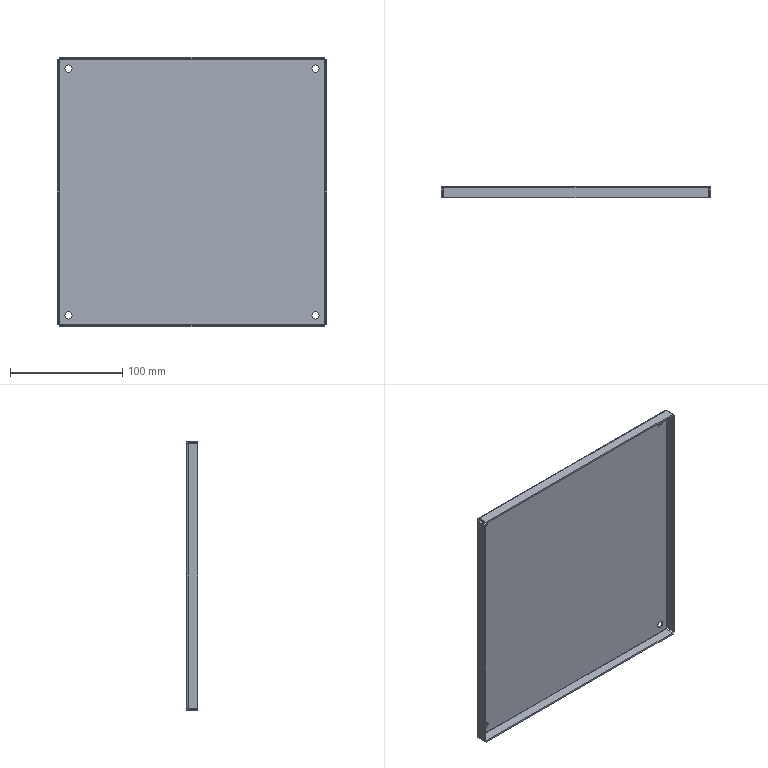Part | SolidWorks | features EdgeFlange 1, FlatPattern 1, ICE 1, SMBaseFlange 1, SheetMetal 1 | 1 solid | 46 faces | box 240.001 x 10 x 240.001 mm | volume 97684 mm3 | plane 22 | cylinder 16 | spline 8 | commonest cylinder face diameters 6.4 x8 0.2 x4 3.2 x4